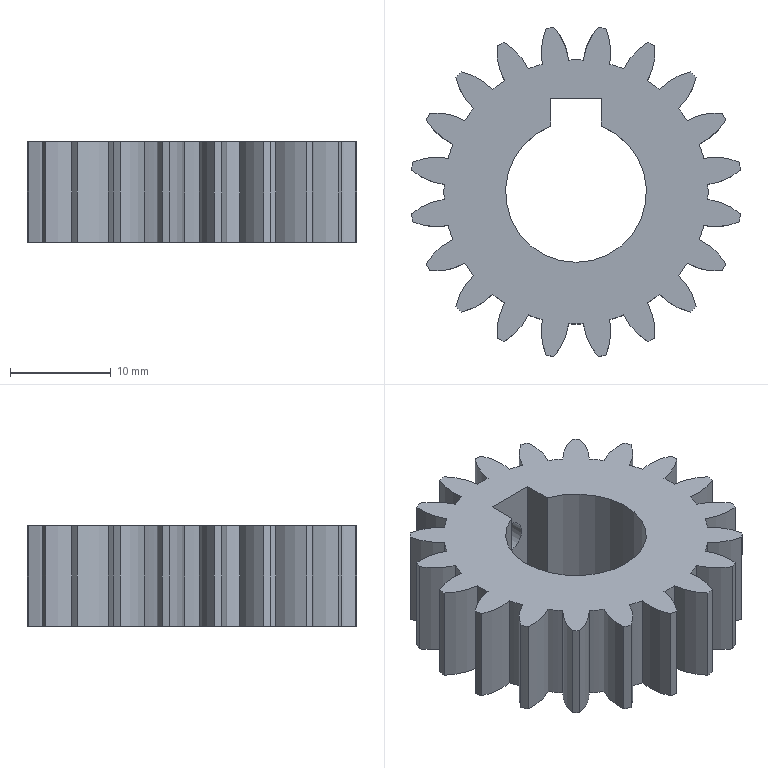Part | NX | features BREP 1 | 1 solid | 88 faces | box 32.708 x 32.708 x 10 mm | volume 5122 mm3 | cylinder 83 | plane 5 | commonest cylinder face diameters 12 x40 26.248 x21 33 x20 3.3 x1 14 x1